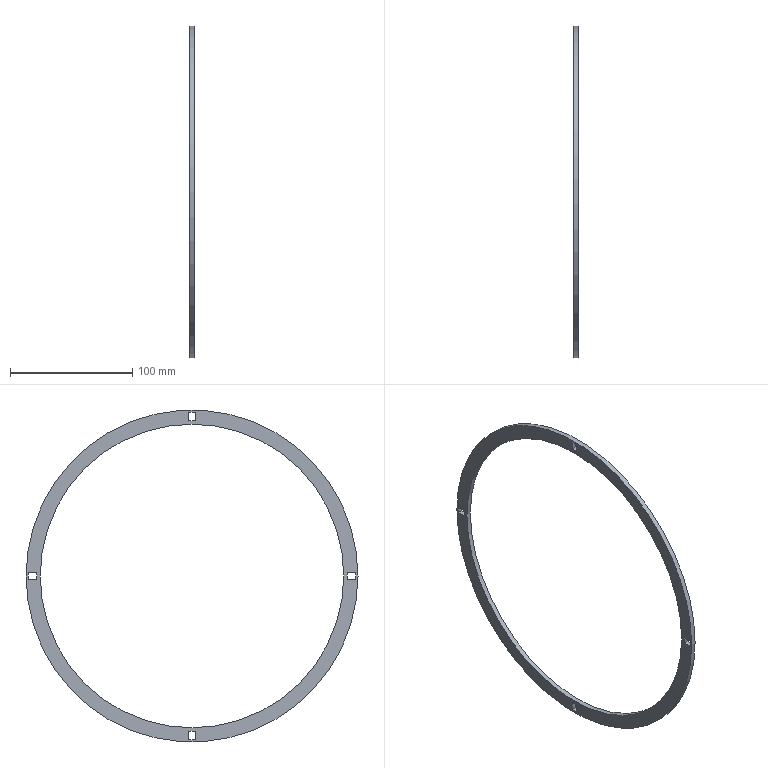Part | STEP file | Part [7] | 1 solid | 20 faces | box 4 x 272.1 x 272.1 mm | volume 37523 mm3 | plane 18 | cylinder 2 | commonest cylinder face diameters 248.83 x1 272.1 x1
STEP:
#1=CARTESIAN_POINT('',(12.,-136.05,0.));
#2=VERTEX_POINT('',#1);
#3=CARTESIAN_POINT('',(12.,0.,0.));
#4=DIRECTION('',(1.,0.,0.));
#5=DIRECTION('',(0.,1.,0.));
#6=AXIS2_PLACEMENT_3D('',#3,#4,#5);
#7=CIRCLE('',#6,136.05);
#8=EDGE_CURVE('',#2,#2,#7,.T.);
#9=ORIENTED_EDGE('',*,*,#8,.T.);
#10=EDGE_LOOP('',(#9));
#11=FACE_BOUND('',#10,.T.);
#12=CARTESIAN_POINT('',(12.,-124.415,0.));
#13=VERTEX_POINT('',#12);
#14=CARTESIAN_POINT('',(12.,0.,0.));
#15=DIRECTION('',(-1.,0.,0.));
#16=DIRECTION('',(0.,1.,0.));
#17=AXIS2_PLACEMENT_3D('',#14,#15,#16);
#18=CIRCLE('',#17,124.415);
#19=EDGE_CURVE('',#13,#13,#18,.T.);
#20=ORIENTED_EDGE('',*,*,#19,.T.);
#21=EDGE_LOOP('',(#20));
#22=FACE_BOUND('',#21,.T.);
#23=CARTESIAN_POINT('',(12.,134.276,-2.5));
#24=VERTEX_POINT('',#23);
#25=CARTESIAN_POINT('',(12.,134.276,2.5));
#26=VERTEX_POINT('',#25);
#27=CARTESIAN_POINT('',(12.,134.276,-2.5));
#28=DIRECTION('',(0.,0.,1.));
#29=VECTOR('',#28,1.);
#30=LINE('',#27,#29);
#31=EDGE_CURVE('',#24,#26,#30,.T.);
#32=ORIENTED_EDGE('',*,*,#31,.F.);
#33=CARTESIAN_POINT('',(12.,127.276,-2.5));
#34=VERTEX_POINT('',#33);
#35=CARTESIAN_POINT('',(12.,127.276,-2.5));
#36=DIRECTION('',(0.,1.,0.));
#37=VECTOR('',#36,1.);
#38=LINE('',#35,#37);
#39=EDGE_CURVE('',#34,#24,#38,.T.);
#40=ORIENTED_EDGE('',*,*,#39,.F.);
#41=CARTESIAN_POINT('',(12.,127.276,2.5));
#42=VERTEX_POINT('',#41);
#43=CARTESIAN_POINT('',(12.,127.276,2.5));
#44=DIRECTION('',(0.,0.,-1.));
#45=VECTOR('',#44,1.);
#46=LINE('',#43,#45);
#47=EDGE_CURVE('',#42,#34,#46,.T.);
#48=ORIENTED_EDGE('',*,*,#47,.F.);
#49=CARTESIAN_POINT('',(12.,134.276,2.5));
#50=DIRECTION('',(0.,-1.,0.));
#51=VECTOR('',#50,1.);
#52=LINE('',#49,#51);
#53=EDGE_CURVE('',#26,#42,#52,.T.);
#54=ORIENTED_EDGE('',*,*,#53,.F.);
#55=EDGE_LOOP('',(#32,#40,#48,#54));
#56=FACE_BOUND('',#55,.T.);
#57=CARTESIAN_POINT('',(12.,-2.5,-134.276));
#58=VERTEX_POINT('',#57);
#59=CARTESIAN_POINT('',(12.,2.5,-134.276));
#60=VERTEX_POINT('',#59);
#61=CARTESIAN_POINT('',(12.,-2.5,-134.276));
#62=DIRECTION('',(0.,1.,0.));
#63=VECTOR('',#62,1.);
#64=LINE('',#61,#63);
#65=EDGE_CURVE('',#58,#60,#64,.T.);
#66=ORIENTED_EDGE('',*,*,#65,.F.);
#67=CARTESIAN_POINT('',(12.,-2.5,-127.276));
#68=VERTEX_POINT('',#67);
#69=CARTESIAN_POINT('',(12.,-2.5,-127.276));
#70=DIRECTION('',(0.,0.,-1.));
#71=VECTOR('',#70,1.);
#72=LINE('',#69,#71);
#73=EDGE_CURVE('',#68,#58,#72,.T.);
#74=ORIENTED_EDGE('',*,*,#73,.F.);
#75=CARTESIAN_POINT('',(12.,2.5,-127.276));
#76=VERTEX_POINT('',#75);
#77=CARTESIAN_POINT('',(12.,2.5,-127.276));
#78=DIRECTION('',(0.,-1.,0.));
#79=VECTOR('',#78,1.);
#80=LINE('',#77,#79);
#81=EDGE_CURVE('',#76,#68,#80,.T.);
#82=ORIENTED_EDGE('',*,*,#81,.F.);
#83=CARTESIAN_POINT('',(12.,2.5,-134.276));
#84=DIRECTION('',(0.,0.,1.));
#85=VECTOR('',#84,1.);
#86=LINE('',#83,#85);
#87=EDGE_CURVE('',#60,#76,#86,.T.);
#88=ORIENTED_EDGE('',*,*,#87,.F.);
#89=EDGE_LOOP('',(#66,#74,#82,#88));
#90=FACE_BOUND('',#89,.T.);
#91=CARTESIAN_POINT('',(12.,-134.276,2.5));
#92=VERTEX_POINT('',#91);
#93=CARTESIAN_POINT('',(12.,-134.276,-2.5));
#94=VERTEX_POINT('',#93);
#95=CARTESIAN_POINT('',(12.,-134.276,2.5));
#96=DIRECTION('',(0.,0.,-1.));
#97=VECTOR('',#96,1.);
#98=LINE('',#95,#97);
#99=EDGE_CURVE('',#92,#94,#98,.T.);
#100=ORIENTED_EDGE('',*,*,#99,.F.);
#101=CARTESIAN_POINT('',(12.,-127.276,2.5));
#102=VERTEX_POINT('',#101);
#103=CARTESIAN_POINT('',(12.,-127.276,2.5));
#104=DIRECTION('',(0.,-1.,0.));
#105=VECTOR('',#104,1.);
#106=LINE('',#103,#105);
#107=EDGE_CURVE('',#102,#92,#106,.T.);
#108=ORIENTED_EDGE('',*,*,#107,.F.);
#109=CARTESIAN_POINT('',(12.,-127.276,-2.5));
#110=VERTEX_POINT('',#109);
#111=CARTESIAN_POINT('',(12.,-127.276,-2.5));
#112=DIRECTION('',(0.,0.,1.));
#113=VECTOR('',#112,1.);
#114=LINE('',#111,#113);
#115=EDGE_CURVE('',#110,#102,#114,.T.);
#116=ORIENTED_EDGE('',*,*,#115,.F.);
#117=CARTESIAN_POINT('',(12.,-134.276,-2.5));
#118=DIRECTION('',(0.,1.,0.));
#119=VECTOR('',#118,1.);
#120=LINE('',#117,#119);
#121=EDGE_CURVE('',#94,#110,#120,.T.);
#122=ORIENTED_EDGE('',*,*,#121,.F.);
#123=EDGE_LOOP('',(#100,#108,#116,#122));
#124=FACE_BOUND('',#123,.T.);
#125=CARTESIAN_POINT('',(12.,2.5,134.276));
#126=VERTEX_POINT('',#125);
#127=CARTESIAN_POINT('',(12.,-2.5,134.276));
#128=VERTEX_POINT('',#127);
#129=CARTESIAN_POINT('',(12.,2.5,134.276));
#130=DIRECTION('',(0.,-1.,0.));
#131=VECTOR('',#130,1.);
#132=LINE('',#129,#131);
#133=EDGE_CURVE('',#126,#128,#132,.T.);
#134=ORIENTED_EDGE('',*,*,#133,.F.);
#135=CARTESIAN_POINT('',(12.,2.5,127.276));
#136=VERTEX_POINT('',#135);
#137=CARTESIAN_POINT('',(12.,2.5,127.276));
#138=DIRECTION('',(0.,0.,1.));
#139=VECTOR('',#138,1.);
#140=LINE('',#137,#139);
#141=EDGE_CURVE('',#136,#126,#140,.T.);
#142=ORIENTED_EDGE('',*,*,#141,.F.);
#143=CARTESIAN_POINT('',(12.,-2.5,127.276));
#144=VERTEX_POINT('',#143);
#145=CARTESIAN_POINT('',(12.,-2.5,127.276));
#146=DIRECTION('',(0.,1.,0.));
#147=VECTOR('',#146,1.);
#148=LINE('',#145,#147);
#149=EDGE_CURVE('',#144,#136,#148,.T.);
#150=ORIENTED_EDGE('',*,*,#149,.F.);
#151=CARTESIAN_POINT('',(12.,-2.5,134.276));
#152=DIRECTION('',(0.,0.,-1.));
#153=VECTOR('',#152,1.);
#154=LINE('',#151,#153);
#155=EDGE_CURVE('',#128,#144,#154,.T.);
#156=ORIENTED_EDGE('',*,*,#155,.F.);
#157=EDGE_LOOP('',(#134,#142,#150,#156));
#158=FACE_BOUND('',#157,.T.);
#159=CARTESIAN_POINT('',(12.,0.,0.));
#160=DIRECTION('',(-1.,0.,0.));
#161=DIRECTION('',(0.,0.,1.));
#162=AXIS2_PLACEMENT_3D('',#159,#160,#161);
#163=PLANE('',#162);
#164=ADVANCED_FACE('',(#11,#22,#56,#90,#124,#158),#163,.F.);
#165=ORIENTED_EDGE('',*,*,#19,.F.);
#166=EDGE_LOOP('',(#165));
#167=FACE_OUTER_BOUND('',#166,.T.);
#168=CARTESIAN_POINT('',(8.,-124.415,0.));
#169=VERTEX_POINT('',#168);
#170=CARTESIAN_POINT('',(8.,0.,0.));
#171=DIRECTION('',(-1.,0.,0.));
#172=DIRECTION('',(0.,1.,0.));
#173=AXIS2_PLACEMENT_3D('',#170,#171,#172);
#174=CIRCLE('',#173,124.415);
#175=EDGE_CURVE('',#169,#169,#174,.T.);
#176=ORIENTED_EDGE('',*,*,#175,.T.);
#177=EDGE_LOOP('',(#176));
#178=FACE_OUTER_BOUND('',#177,.T.);
#179=CARTESIAN_POINT('',(12.2,0.,0.));
#180=DIRECTION('',(-1.,0.,0.));
#181=DIRECTION('',(0.,-1.,0.));
#182=AXIS2_PLACEMENT_3D('',#179,#180,#181);
#183=CYLINDRICAL_SURFACE('',#182,124.415);
#184=ADVANCED_FACE('',(#167,#178),#183,.F.);
#185=CARTESIAN_POINT('',(8.,-136.05,0.));
#186=VERTEX_POINT('',#185);
#187=CARTESIAN_POINT('',(8.,0.,0.));
#188=DIRECTION('',(-1.,0.,0.));
#189=DIRECTION('',(0.,1.,0.));
#190=AXIS2_PLACEMENT_3D('',#187,#188,#189);
#191=CIRCLE('',#190,136.05);
#192=EDGE_CURVE('',#186,#186,#191,.T.);
#193=ORIENTED_EDGE('',*,*,#192,.T.);
#194=EDGE_LOOP('',(#193));
#195=FACE_BOUND('',#194,.T.);
#196=ORIENTED_EDGE('',*,*,#175,.F.);
#197=EDGE_LOOP('',(#196));
#198=FACE_BOUND('',#197,.T.);
#199=CARTESIAN_POINT('',(8.,127.276,2.5));
#200=VERTEX_POINT('',#199);
#201=CARTESIAN_POINT('',(8.,127.276,-2.5));
#202=VERTEX_POINT('',#201);
#203=CARTESIAN_POINT('',(8.,127.276,2.5));
#204=DIRECTION('',(0.,0.,-1.));
#205=VECTOR('',#204,1.);
#206=LINE('',#203,#205);
#207=EDGE_CURVE('',#200,#202,#206,.T.);
#208=ORIENTED_EDGE('',*,*,#207,.T.);
#209=CARTESIAN_POINT('',(8.,134.276,-2.5));
#210=VERTEX_POINT('',#209);
#211=CARTESIAN_POINT('',(8.,127.276,-2.5));
#212=DIRECTION('',(0.,1.,0.));
#213=VECTOR('',#212,1.);
#214=LINE('',#211,#213);
#215=EDGE_CURVE('',#202,#210,#214,.T.);
#216=ORIENTED_EDGE('',*,*,#215,.T.);
#217=CARTESIAN_POINT('',(8.,134.276,2.5));
#218=VERTEX_POINT('',#217);
#219=CARTESIAN_POINT('',(8.,134.276,-2.5));
#220=DIRECTION('',(0.,0.,1.));
#221=VECTOR('',#220,1.);
#222=LINE('',#219,#221);
#223=EDGE_CURVE('',#210,#218,#222,.T.);
#224=ORIENTED_EDGE('',*,*,#223,.T.);
#225=CARTESIAN_POINT('',(8.,134.276,2.5));
#226=DIRECTION('',(0.,-1.,0.));
#227=VECTOR('',#226,1.);
#228=LINE('',#225,#227);
#229=EDGE_CURVE('',#218,#200,#228,.T.);
#230=ORIENTED_EDGE('',*,*,#229,.T.);
#231=EDGE_LOOP('',(#208,#216,#224,#230));
#232=FACE_BOUND('',#231,.T.);
#233=CARTESIAN_POINT('',(8.,2.5,-127.276));
#234=VERTEX_POINT('',#233);
#235=CARTESIAN_POINT('',(8.,-2.5,-127.276));
#236=VERTEX_POINT('',#235);
#237=CARTESIAN_POINT('',(8.,2.5,-127.276));
#238=DIRECTION('',(0.,-1.,0.));
#239=VECTOR('',#238,1.);
#240=LINE('',#237,#239);
#241=EDGE_CURVE('',#234,#236,#240,.T.);
#242=ORIENTED_EDGE('',*,*,#241,.T.);
#243=CARTESIAN_POINT('',(8.,-2.5,-134.276));
#244=VERTEX_POINT('',#243);
#245=CARTESIAN_POINT('',(8.,-2.5,-127.276));
#246=DIRECTION('',(0.,0.,-1.));
#247=VECTOR('',#246,1.);
#248=LINE('',#245,#247);
#249=EDGE_CURVE('',#236,#244,#248,.T.);
#250=ORIENTED_EDGE('',*,*,#249,.T.);
#251=CARTESIAN_POINT('',(8.,2.5,-134.276));
#252=VERTEX_POINT('',#251);
#253=CARTESIAN_POINT('',(8.,-2.5,-134.276));
#254=DIRECTION('',(0.,1.,0.));
#255=VECTOR('',#254,1.);
#256=LINE('',#253,#255);
#257=EDGE_CURVE('',#244,#252,#256,.T.);
#258=ORIENTED_EDGE('',*,*,#257,.T.);
#259=CARTESIAN_POINT('',(8.,2.5,-134.276));
#260=DIRECTION('',(0.,0.,1.));
#261=VECTOR('',#260,1.);
#262=LINE('',#259,#261);
#263=EDGE_CURVE('',#252,#234,#262,.T.);
#264=ORIENTED_EDGE('',*,*,#263,.T.);
#265=EDGE_LOOP('',(#242,#250,#258,#264));
#266=FACE_BOUND('',#265,.T.);
#267=CARTESIAN_POINT('',(8.,-127.276,-2.5));
#268=VERTEX_POINT('',#267);
#269=CARTESIAN_POINT('',(8.,-127.276,2.5));
#270=VERTEX_POINT('',#269);
#271=CARTESIAN_POINT('',(8.,-127.276,-2.5));
#272=DIRECTION('',(0.,0.,1.));
#273=VECTOR('',#272,1.);
#274=LINE('',#271,#273);
#275=EDGE_CURVE('',#268,#270,#274,.T.);
#276=ORIENTED_EDGE('',*,*,#275,.T.);
#277=CARTESIAN_POINT('',(8.,-134.276,2.5));
#278=VERTEX_POINT('',#277);
#279=CARTESIAN_POINT('',(8.,-127.276,2.5));
#280=DIRECTION('',(0.,-1.,0.));
#281=VECTOR('',#280,1.);
#282=LINE('',#279,#281);
#283=EDGE_CURVE('',#270,#278,#282,.T.);
#284=ORIENTED_EDGE('',*,*,#283,.T.);
#285=CARTESIAN_POINT('',(8.,-134.276,-2.5));
#286=VERTEX_POINT('',#285);
#287=CARTESIAN_POINT('',(8.,-134.276,2.5));
#288=DIRECTION('',(0.,0.,-1.));
#289=VECTOR('',#288,1.);
#290=LINE('',#287,#289);
#291=EDGE_CURVE('',#278,#286,#290,.T.);
#292=ORIENTED_EDGE('',*,*,#291,.T.);
#293=CARTESIAN_POINT('',(8.,-134.276,-2.5));
#294=DIRECTION('',(0.,1.,0.));
#295=VECTOR('',#294,1.);
#296=LINE('',#293,#295);
#297=EDGE_CURVE('',#286,#268,#296,.T.);
#298=ORIENTED_EDGE('',*,*,#297,.T.);
#299=EDGE_LOOP('',(#276,#284,#292,#298));
#300=FACE_BOUND('',#299,.T.);
#301=CARTESIAN_POINT('',(8.,-2.5,127.276));
#302=VERTEX_POINT('',#301);
#303=CARTESIAN_POINT('',(8.,2.5,127.276));
#304=VERTEX_POINT('',#303);
#305=CARTESIAN_POINT('',(8.,-2.5,127.276));
#306=DIRECTION('',(0.,1.,0.));
#307=VECTOR('',#306,1.);
#308=LINE('',#305,#307);
#309=EDGE_CURVE('',#302,#304,#308,.T.);
#310=ORIENTED_EDGE('',*,*,#309,.T.);
#311=CARTESIAN_POINT('',(8.,2.5,134.276));
#312=VERTEX_POINT('',#311);
#313=CARTESIAN_POINT('',(8.,2.5,127.276));
#314=DIRECTION('',(0.,0.,1.));
#315=VECTOR('',#314,1.);
#316=LINE('',#313,#315);
#317=EDGE_CURVE('',#304,#312,#316,.T.);
#318=ORIENTED_EDGE('',*,*,#317,.T.);
#319=CARTESIAN_POINT('',(8.,-2.5,134.276));
#320=VERTEX_POINT('',#319);
#321=CARTESIAN_POINT('',(8.,2.5,134.276));
#322=DIRECTION('',(0.,-1.,0.));
#323=VECTOR('',#322,1.);
#324=LINE('',#321,#323);
#325=EDGE_CURVE('',#312,#320,#324,.T.);
#326=ORIENTED_EDGE('',*,*,#325,.T.);
#327=CARTESIAN_POINT('',(8.,-2.5,134.276));
#328=DIRECTION('',(0.,0.,-1.));
#329=VECTOR('',#328,1.);
#330=LINE('',#327,#329);
#331=EDGE_CURVE('',#320,#302,#330,.T.);
#332=ORIENTED_EDGE('',*,*,#331,.T.);
#333=EDGE_LOOP('',(#310,#318,#326,#332));
#334=FACE_BOUND('',#333,.T.);
#335=CARTESIAN_POINT('',(8.,0.,0.));
#336=DIRECTION('',(-1.,0.,0.));
#337=DIRECTION('',(0.,0.,1.));
#338=AXIS2_PLACEMENT_3D('',#335,#336,#337);
#339=PLANE('',#338);
#340=ADVANCED_FACE('',(#195,#198,#232,#266,#300,#334),#339,.T.);
#341=ORIENTED_EDGE('',*,*,#8,.F.);
#342=EDGE_LOOP('',(#341));
#343=FACE_OUTER_BOUND('',#342,.T.);
#344=ORIENTED_EDGE('',*,*,#192,.F.);
#345=EDGE_LOOP('',(#344));
#346=FACE_OUTER_BOUND('',#345,.T.);
#347=CARTESIAN_POINT('',(12.2,0.,0.));
#348=DIRECTION('',(-1.,0.,0.));
#349=DIRECTION('',(0.,-1.,0.));
#350=AXIS2_PLACEMENT_3D('',#347,#348,#349);
#351=CYLINDRICAL_SURFACE('',#350,136.05);
#352=ADVANCED_FACE('',(#343,#346),#351,.T.);
#353=CARTESIAN_POINT('',(12.,127.276,2.5));
#354=DIRECTION('',(-1.,0.,0.));
#355=VECTOR('',#354,1.);
#356=LINE('',#353,#355);
#357=EDGE_CURVE('',#42,#200,#356,.T.);
#358=ORIENTED_EDGE('',*,*,#357,.T.);
#359=ORIENTED_EDGE('',*,*,#229,.F.);
#360=CARTESIAN_POINT('',(12.,134.276,2.5));
#361=DIRECTION('',(-1.,0.,0.));
#362=VECTOR('',#361,1.);
#363=LINE('',#360,#362);
#364=EDGE_CURVE('',#26,#218,#363,.T.);
#365=ORIENTED_EDGE('',*,*,#364,.F.);
#366=ORIENTED_EDGE('',*,*,#53,.T.);
#367=EDGE_LOOP('',(#358,#359,#365,#366));
#368=FACE_BOUND('',#367,.T.);
#369=CARTESIAN_POINT('',(12.,134.276,2.5));
#370=DIRECTION('',(0.,0.,1.));
#371=DIRECTION('',(1.,0.,0.));
#372=AXIS2_PLACEMENT_3D('',#369,#370,#371);
#373=PLANE('',#372);
#374=ADVANCED_FACE('',(#368),#373,.F.);
#375=ORIENTED_EDGE('',*,*,#364,.T.);
#376=ORIENTED_EDGE('',*,*,#223,.F.);
#377=CARTESIAN_POINT('',(12.,134.276,-2.5));
#378=DIRECTION('',(-1.,0.,0.));
#379=VECTOR('',#378,1.);
#380=LINE('',#377,#379);
#381=EDGE_CURVE('',#24,#210,#380,.T.);
#382=ORIENTED_EDGE('',*,*,#381,.F.);
#383=ORIENTED_EDGE('',*,*,#31,.T.);
#384=EDGE_LOOP('',(#375,#376,#382,#383));
#385=FACE_BOUND('',#384,.T.);
#386=CARTESIAN_POINT('',(12.,134.276,-2.5));
#387=DIRECTION('',(0.,1.,0.));
#388=DIRECTION('',(1.,0.,0.));
#389=AXIS2_PLACEMENT_3D('',#386,#387,#388);
#390=PLANE('',#389);
#391=ADVANCED_FACE('',(#385),#390,.F.);
#392=ORIENTED_EDGE('',*,*,#381,.T.);
#393=ORIENTED_EDGE('',*,*,#215,.F.);
#394=CARTESIAN_POINT('',(12.,127.276,-2.5));
#395=DIRECTION('',(-1.,0.,0.));
#396=VECTOR('',#395,1.);
#397=LINE('',#394,#396);
#398=EDGE_CURVE('',#34,#202,#397,.T.);
#399=ORIENTED_EDGE('',*,*,#398,.F.);
#400=ORIENTED_EDGE('',*,*,#39,.T.);
#401=EDGE_LOOP('',(#392,#393,#399,#400));
#402=FACE_BOUND('',#401,.T.);
#403=CARTESIAN_POINT('',(12.,127.276,-2.5));
#404=DIRECTION('',(0.,0.,-1.));
#405=DIRECTION('',(0.,-1.,0.));
#406=AXIS2_PLACEMENT_3D('',#403,#404,#405);
#407=PLANE('',#406);
#408=ADVANCED_FACE('',(#402),#407,.F.);
#409=ORIENTED_EDGE('',*,*,#398,.T.);
#410=ORIENTED_EDGE('',*,*,#207,.F.);
#411=ORIENTED_EDGE('',*,*,#357,.F.);
#412=ORIENTED_EDGE('',*,*,#47,.T.);
#413=EDGE_LOOP('',(#409,#410,#411,#412));
#414=FACE_BOUND('',#413,.T.);
#415=CARTESIAN_POINT('',(12.,127.276,2.5));
#416=DIRECTION('',(0.,-1.,0.));
#417=DIRECTION('',(0.,0.,-1.));
#418=AXIS2_PLACEMENT_3D('',#415,#416,#417);
#419=PLANE('',#418);
#420=ADVANCED_FACE('',(#414),#419,.F.);
#421=CARTESIAN_POINT('',(12.,2.5,-127.276));
#422=DIRECTION('',(-1.,0.,0.));
#423=VECTOR('',#422,1.);
#424=LINE('',#421,#423);
#425=EDGE_CURVE('',#76,#234,#424,.T.);
#426=ORIENTED_EDGE('',*,*,#425,.T.);
#427=ORIENTED_EDGE('',*,*,#263,.F.);
#428=CARTESIAN_POINT('',(12.,2.5,-134.276));
#429=DIRECTION('',(-1.,0.,0.));
#430=VECTOR('',#429,1.);
#431=LINE('',#428,#430);
#432=EDGE_CURVE('',#60,#252,#431,.T.);
#433=ORIENTED_EDGE('',*,*,#432,.F.);
#434=ORIENTED_EDGE('',*,*,#87,.T.);
#435=EDGE_LOOP('',(#426,#427,#433,#434));
#436=FACE_BOUND('',#435,.T.);
#437=CARTESIAN_POINT('',(12.,2.5,-134.276));
#438=DIRECTION('',(0.,1.,0.));
#439=DIRECTION('',(1.,0.,0.));
#440=AXIS2_PLACEMENT_3D('',#437,#438,#439);
#441=PLANE('',#440);
#442=ADVANCED_FACE('',(#436),#441,.F.);
#443=ORIENTED_EDGE('',*,*,#432,.T.);
#444=ORIENTED_EDGE('',*,*,#257,.F.);
#445=CARTESIAN_POINT('',(12.,-2.5,-134.276));
#446=DIRECTION('',(-1.,0.,0.));
#447=VECTOR('',#446,1.);
#448=LINE('',#445,#447);
#449=EDGE_CURVE('',#58,#244,#448,.T.);
#450=ORIENTED_EDGE('',*,*,#449,.F.);
#451=ORIENTED_EDGE('',*,*,#65,.T.);
#452=EDGE_LOOP('',(#443,#444,#450,#451));
#453=FACE_BOUND('',#452,.T.);
#454=CARTESIAN_POINT('',(12.,-2.5,-134.276));
#455=DIRECTION('',(0.,0.,-1.));
#456=DIRECTION('',(0.,-1.,0.));
#457=AXIS2_PLACEMENT_3D('',#454,#455,#456);
#458=PLANE('',#457);
#459=ADVANCED_FACE('',(#453),#458,.F.);
#460=ORIENTED_EDGE('',*,*,#449,.T.);
#461=ORIENTED_EDGE('',*,*,#249,.F.);
#462=CARTESIAN_POINT('',(12.,-2.5,-127.276));
#463=DIRECTION('',(-1.,0.,0.));
#464=VECTOR('',#463,1.);
#465=LINE('',#462,#464);
#466=EDGE_CURVE('',#68,#236,#465,.T.);
#467=ORIENTED_EDGE('',*,*,#466,.F.);
#468=ORIENTED_EDGE('',*,*,#73,.T.);
#469=EDGE_LOOP('',(#460,#461,#467,#468));
#470=FACE_BOUND('',#469,.T.);
#471=CARTESIAN_POINT('',(12.,-2.5,-127.276));
#472=DIRECTION('',(0.,-1.,0.));
#473=DIRECTION('',(0.,0.,-1.));
#474=AXIS2_PLACEMENT_3D('',#471,#472,#473);
#475=PLANE('',#474);
#476=ADVANCED_FACE('',(#470),#475,.F.);
#477=ORIENTED_EDGE('',*,*,#466,.T.);
#478=ORIENTED_EDGE('',*,*,#241,.F.);
#479=ORIENTED_EDGE('',*,*,#425,.F.);
#480=ORIENTED_EDGE('',*,*,#81,.T.);
#481=EDGE_LOOP('',(#477,#478,#479,#480));
#482=FACE_BOUND('',#481,.T.);
#483=CARTESIAN_POINT('',(12.,2.5,-127.276));
#484=DIRECTION('',(0.,0.,1.));
#485=DIRECTION('',(1.,0.,0.));
#486=AXIS2_PLACEMENT_3D('',#483,#484,#485);
#487=PLANE('',#486);
#488=ADVANCED_FACE('',(#482),#487,.F.);
#489=CARTESIAN_POINT('',(12.,-127.276,-2.5));
#490=DIRECTION('',(-1.,0.,0.));
#491=VECTOR('',#490,1.);
#492=LINE('',#489,#491);
#493=EDGE_CURVE('',#110,#268,#492,.T.);
#494=ORIENTED_EDGE('',*,*,#493,.T.);
#495=ORIENTED_EDGE('',*,*,#297,.F.);
#496=CARTESIAN_POINT('',(12.,-134.276,-2.5));
#497=DIRECTION('',(-1.,0.,0.));
#498=VECTOR('',#497,1.);
#499=LINE('',#496,#498);
#500=EDGE_CURVE('',#94,#286,#499,.T.);
#501=ORIENTED_EDGE('',*,*,#500,.F.);
#502=ORIENTED_EDGE('',*,*,#121,.T.);
#503=EDGE_LOOP('',(#494,#495,#501,#502));
#504=FACE_BOUND('',#503,.T.);
#505=CARTESIAN_POINT('',(12.,-134.276,-2.5));
#506=DIRECTION('',(0.,0.,-1.));
#507=DIRECTION('',(0.,-1.,0.));
#508=AXIS2_PLACEMENT_3D('',#505,#506,#507);
#509=PLANE('',#508);
#510=ADVANCED_FACE('',(#504),#509,.F.);
#511=ORIENTED_EDGE('',*,*,#500,.T.);
#512=ORIENTED_EDGE('',*,*,#291,.F.);
#513=CARTESIAN_POINT('',(12.,-134.276,2.5));
#514=DIRECTION('',(-1.,0.,0.));
#515=VECTOR('',#514,1.);
#516=LINE('',#513,#515);
#517=EDGE_CURVE('',#92,#278,#516,.T.);
#518=ORIENTED_EDGE('',*,*,#517,.F.);
#519=ORIENTED_EDGE('',*,*,#99,.T.);
#520=EDGE_LOOP('',(#511,#512,#518,#519));
#521=FACE_BOUND('',#520,.T.);
#522=CARTESIAN_POINT('',(12.,-134.276,2.5));
#523=DIRECTION('',(0.,-1.,0.));
#524=DIRECTION('',(0.,0.,-1.));
#525=AXIS2_PLACEMENT_3D('',#522,#523,#524);
#526=PLANE('',#525);
#527=ADVANCED_FACE('',(#521),#526,.F.);
#528=ORIENTED_EDGE('',*,*,#517,.T.);
#529=ORIENTED_EDGE('',*,*,#283,.F.);
#530=CARTESIAN_POINT('',(12.,-127.276,2.5));
#531=DIRECTION('',(-1.,0.,0.));
#532=VECTOR('',#531,1.);
#533=LINE('',#530,#532);
#534=EDGE_CURVE('',#102,#270,#533,.T.);
#535=ORIENTED_EDGE('',*,*,#534,.F.);
#536=ORIENTED_EDGE('',*,*,#107,.T.);
#537=EDGE_LOOP('',(#528,#529,#535,#536));
#538=FACE_BOUND('',#537,.T.);
#539=CARTESIAN_POINT('',(12.,-127.276,2.5));
#540=DIRECTION('',(0.,0.,1.));
#541=DIRECTION('',(1.,0.,0.));
#542=AXIS2_PLACEMENT_3D('',#539,#540,#541);
#543=PLANE('',#542);
#544=ADVANCED_FACE('',(#538),#543,.F.);
#545=ORIENTED_EDGE('',*,*,#534,.T.);
#546=ORIENTED_EDGE('',*,*,#275,.F.);
#547=ORIENTED_EDGE('',*,*,#493,.F.);
#548=ORIENTED_EDGE('',*,*,#115,.T.);
#549=EDGE_LOOP('',(#545,#546,#547,#548));
#550=FACE_BOUND('',#549,.T.);
#551=CARTESIAN_POINT('',(12.,-127.276,-2.5));
#552=DIRECTION('',(0.,1.,0.));
#553=DIRECTION('',(1.,0.,0.));
#554=AXIS2_PLACEMENT_3D('',#551,#552,#553);
#555=PLANE('',#554);
#556=ADVANCED_FACE('',(#550),#555,.F.);
#557=CARTESIAN_POINT('',(12.,-2.5,127.276));
#558=DIRECTION('',(-1.,0.,0.));
#559=VECTOR('',#558,1.);
#560=LINE('',#557,#559);
#561=EDGE_CURVE('',#144,#302,#560,.T.);
#562=ORIENTED_EDGE('',*,*,#561,.T.);
#563=ORIENTED_EDGE('',*,*,#331,.F.);
#564=CARTESIAN_POINT('',(12.,-2.5,134.276));
#565=DIRECTION('',(-1.,0.,0.));
#566=VECTOR('',#565,1.);
#567=LINE('',#564,#566);
#568=EDGE_CURVE('',#128,#320,#567,.T.);
#569=ORIENTED_EDGE('',*,*,#568,.F.);
#570=ORIENTED_EDGE('',*,*,#155,.T.);
#571=EDGE_LOOP('',(#562,#563,#569,#570));
#572=FACE_BOUND('',#571,.T.);
#573=CARTESIAN_POINT('',(12.,-2.5,134.276));
#574=DIRECTION('',(0.,-1.,0.));
#575=DIRECTION('',(0.,0.,-1.));
#576=AXIS2_PLACEMENT_3D('',#573,#574,#575);
#577=PLANE('',#576);
#578=ADVANCED_FACE('',(#572),#577,.F.);
#579=ORIENTED_EDGE('',*,*,#568,.T.);
#580=ORIENTED_EDGE('',*,*,#325,.F.);
#581=CARTESIAN_POINT('',(12.,2.5,134.276));
#582=DIRECTION('',(-1.,0.,0.));
#583=VECTOR('',#582,1.);
#584=LINE('',#581,#583);
#585=EDGE_CURVE('',#126,#312,#584,.T.);
#586=ORIENTED_EDGE('',*,*,#585,.F.);
#587=ORIENTED_EDGE('',*,*,#133,.T.);
#588=EDGE_LOOP('',(#579,#580,#586,#587));
#589=FACE_BOUND('',#588,.T.);
#590=CARTESIAN_POINT('',(12.,2.5,134.276));
#591=DIRECTION('',(0.,0.,1.));
#592=DIRECTION('',(1.,0.,0.));
#593=AXIS2_PLACEMENT_3D('',#590,#591,#592);
#594=PLANE('',#593);
#595=ADVANCED_FACE('',(#589),#594,.F.);
#596=ORIENTED_EDGE('',*,*,#585,.T.);
#597=ORIENTED_EDGE('',*,*,#317,.F.);
#598=CARTESIAN_POINT('',(12.,2.5,127.276));
#599=DIRECTION('',(-1.,0.,0.));
#600=VECTOR('',#599,1.);
#601=LINE('',#598,#600);
#602=EDGE_CURVE('',#136,#304,#601,.T.);
#603=ORIENTED_EDGE('',*,*,#602,.F.);
#604=ORIENTED_EDGE('',*,*,#141,.T.);
#605=EDGE_LOOP('',(#596,#597,#603,#604));
#606=FACE_BOUND('',#605,.T.);
#607=CARTESIAN_POINT('',(12.,2.5,127.276));
#608=DIRECTION('',(0.,1.,0.));
#609=DIRECTION('',(1.,0.,0.));
#610=AXIS2_PLACEMENT_3D('',#607,#608,#609);
#611=PLANE('',#610);
#612=ADVANCED_FACE('',(#606),#611,.F.);
#613=ORIENTED_EDGE('',*,*,#602,.T.);
#614=ORIENTED_EDGE('',*,*,#309,.F.);
#615=ORIENTED_EDGE('',*,*,#561,.F.);
#616=ORIENTED_EDGE('',*,*,#149,.T.);
#617=EDGE_LOOP('',(#613,#614,#615,#616));
#618=FACE_BOUND('',#617,.T.);
#619=CARTESIAN_POINT('',(12.,-2.5,127.276));
#620=DIRECTION('',(0.,0.,-1.));
#621=DIRECTION('',(0.,-1.,0.));
#622=AXIS2_PLACEMENT_3D('',#619,#620,#621);
#623=PLANE('',#622);
#624=ADVANCED_FACE('',(#618),#623,.F.);
#625=CLOSED_SHELL('',(#164,#184,#340,#352,#374,#391,#408,#420,#442,#459,#476,#488,#510,#527,#544,#556,#578,#595,#612,#624));
#626=MANIFOLD_SOLID_BREP('',#625);
#627=(LENGTH_UNIT()NAMED_UNIT(*)SI_UNIT(.MILLI.,.METRE.));
#628=UNCERTAINTY_MEASURE_WITH_UNIT(LENGTH_MEASURE(0.00001),#627,'','');
#629=(NAMED_UNIT(*)PLANE_ANGLE_UNIT()SI_UNIT($,.RADIAN.));
#630=(NAMED_UNIT(*)SI_UNIT($,.STERADIAN.)SOLID_ANGLE_UNIT());
#631=(GEOMETRIC_REPRESENTATION_CONTEXT(3)GLOBAL_UNCERTAINTY_ASSIGNED_CONTEXT((#628))GLOBAL_UNIT_ASSIGNED_CONTEXT((#627,#629,#630))REPRESENTATION_CONTEXT('',''));
#632=ADVANCED_BREP_SHAPE_REPRESENTATION('',(#626),#631);